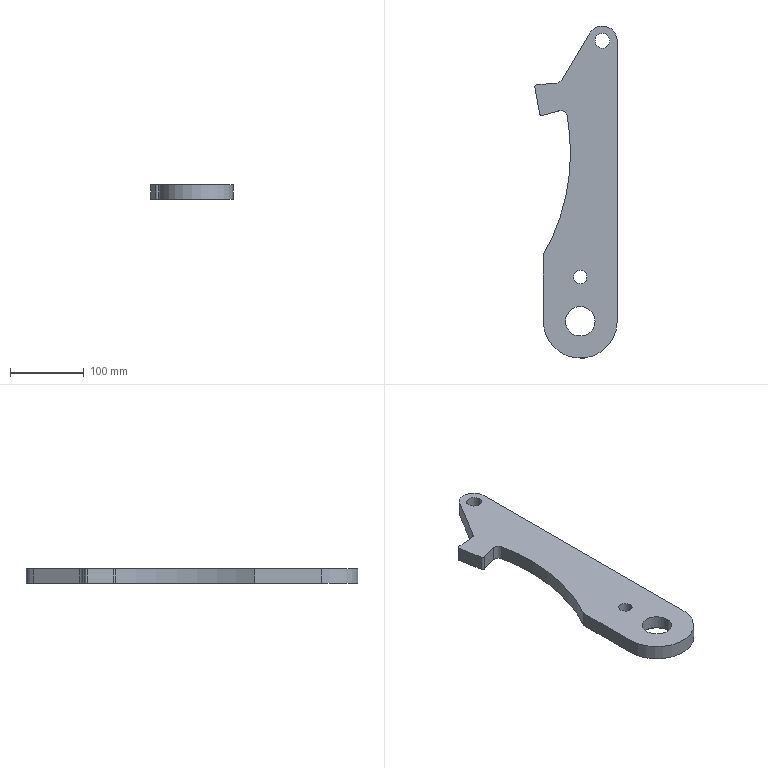Part | SolidWorks | features Fillet 2, Chamfer 1, Extrusion 1 | 1 solid | 24 faces | box 111.471 x 450 x 20 mm | volume 668870 mm3 | cylinder 14 | plane 8 | cone 2 | commonest cylinder face diameters 6 x3 20 x3 40 x3 18 x2 16 x1 100 x1
STEP:
#1=CARTESIAN_POINT('',(20.,0.,2.5));
#2=VERTEX_POINT('',#1);
#3=CARTESIAN_POINT('',(-20.,0.,2.5));
#4=VERTEX_POINT('',#3);
#5=CARTESIAN_POINT('',(0.,0.,2.5));
#6=DIRECTION('',(0.,0.,-1.));
#7=DIRECTION('',(1.,0.,0.));
#8=AXIS2_PLACEMENT_3D('',#5,#6,#7);
#9=CIRCLE('',#8,20.);
#10=EDGE_CURVE('',#2,#4,#9,.T.);
#11=ORIENTED_EDGE('',*,*,#10,.F.);
#12=CARTESIAN_POINT('',(22.5,0.,0.));
#13=VERTEX_POINT('',#12);
#14=CARTESIAN_POINT('',(22.5,0.,0.));
#15=DIRECTION('',(0.7071,0.,-0.7071));
#16=VECTOR('',#15,1000.);
#17=LINE('',#14,#16);
#18=EDGE_CURVE('',#2,#13,#17,.T.);
#19=ORIENTED_EDGE('',*,*,#18,.T.);
#20=CARTESIAN_POINT('',(-22.5,0.,0.));
#21=VERTEX_POINT('',#20);
#22=CARTESIAN_POINT('',(0.,0.,0.));
#23=DIRECTION('',(0.,0.,1.));
#24=DIRECTION('',(1.,0.,0.));
#25=AXIS2_PLACEMENT_3D('',#22,#23,#24);
#26=CIRCLE('',#25,22.5);
#27=EDGE_CURVE('',#21,#13,#26,.T.);
#28=ORIENTED_EDGE('',*,*,#27,.F.);
#29=CARTESIAN_POINT('',(-22.5,0.,0.));
#30=DIRECTION('',(-0.7071,0.,-0.7071));
#31=VECTOR('',#30,1000.);
#32=LINE('',#29,#31);
#33=EDGE_CURVE('',#4,#21,#32,.T.);
#34=ORIENTED_EDGE('',*,*,#33,.F.);
#35=EDGE_LOOP('',(#11,#19,#28,#34));
#36=FACE_OUTER_BOUND('',#35,.T.);
#37=CARTESIAN_POINT('',(0.,0.,0.));
#38=DIRECTION('',(0.,0.,-1.));
#39=DIRECTION('',(-1.,0.,0.));
#40=AXIS2_PLACEMENT_3D('',#37,#38,#39);
#41=CONICAL_SURFACE('',#40,22.5,0.7854);
#42=ADVANCED_FACE('',(#36),#41,.F.);
#43=CARTESIAN_POINT('',(-61.471,317.304,20.));
#44=VERTEX_POINT('',#43);
#45=CARTESIAN_POINT('',(-61.424,316.777,20.));
#46=VERTEX_POINT('',#45);
#47=CARTESIAN_POINT('',(-58.471,317.304,20.));
#48=DIRECTION('',(0.,0.,1.));
#49=DIRECTION('',(1.,0.,0.));
#50=AXIS2_PLACEMENT_3D('',#47,#48,#49);
#51=CIRCLE('',#50,3.);
#52=EDGE_CURVE('',#44,#46,#51,.T.);
#53=ORIENTED_EDGE('',*,*,#52,.F.);
#54=CARTESIAN_POINT('',(-61.471,317.304,0.));
#55=VERTEX_POINT('',#54);
#56=CARTESIAN_POINT('',(-61.471,317.304,20.));
#57=DIRECTION('',(0.,0.,-1.));
#58=VECTOR('',#57,1000.);
#59=LINE('',#56,#58);
#60=EDGE_CURVE('',#44,#55,#59,.T.);
#61=ORIENTED_EDGE('',*,*,#60,.T.);
#62=CARTESIAN_POINT('',(-61.424,316.777,0.));
#63=VERTEX_POINT('',#62);
#64=CARTESIAN_POINT('',(-58.471,317.304,0.));
#65=DIRECTION('',(0.,0.,-1.));
#66=DIRECTION('',(1.,0.,0.));
#67=AXIS2_PLACEMENT_3D('',#64,#65,#66);
#68=CIRCLE('',#67,3.);
#69=EDGE_CURVE('',#63,#55,#68,.T.);
#70=ORIENTED_EDGE('',*,*,#69,.F.);
#71=CARTESIAN_POINT('',(-61.424,316.777,20.));
#72=DIRECTION('',(0.,0.,-1.));
#73=VECTOR('',#72,1000.);
#74=LINE('',#71,#73);
#75=EDGE_CURVE('',#46,#63,#74,.T.);
#76=ORIENTED_EDGE('',*,*,#75,.F.);
#77=EDGE_LOOP('',(#53,#61,#70,#76));
#78=FACE_OUTER_BOUND('',#77,.T.);
#79=CARTESIAN_POINT('',(-58.471,317.304,20.));
#80=DIRECTION('',(0.,0.,-1.));
#81=DIRECTION('',(-1.,0.,0.));
#82=AXIS2_PLACEMENT_3D('',#79,#80,#81);
#83=CYLINDRICAL_SURFACE('',#82,3.);
#84=ADVANCED_FACE('',(#78),#83,.T.);
#85=CARTESIAN_POINT('',(-20.,0.,20.));
#86=VERTEX_POINT('',#85);
#87=CARTESIAN_POINT('',(20.,0.,20.));
#88=VERTEX_POINT('',#87);
#89=CARTESIAN_POINT('',(0.,0.,20.));
#90=DIRECTION('',(0.,0.,1.));
#91=DIRECTION('',(1.,0.,0.));
#92=AXIS2_PLACEMENT_3D('',#89,#90,#91);
#93=CIRCLE('',#92,20.);
#94=EDGE_CURVE('',#86,#88,#93,.T.);
#95=ORIENTED_EDGE('',*,*,#94,.T.);
#96=CARTESIAN_POINT('',(20.,0.,20.));
#97=DIRECTION('',(0.,0.,-1.));
#98=VECTOR('',#97,1000.);
#99=LINE('',#96,#98);
#100=EDGE_CURVE('',#88,#2,#99,.T.);
#101=ORIENTED_EDGE('',*,*,#100,.T.);
#102=ORIENTED_EDGE('',*,*,#10,.T.);
#103=CARTESIAN_POINT('',(-20.,0.,20.));
#104=DIRECTION('',(0.,0.,-1.));
#105=VECTOR('',#104,1000.);
#106=LINE('',#103,#105);
#107=EDGE_CURVE('',#86,#4,#106,.T.);
#108=ORIENTED_EDGE('',*,*,#107,.F.);
#109=EDGE_LOOP('',(#95,#101,#102,#108));
#110=FACE_OUTER_BOUND('',#109,.T.);
#111=CARTESIAN_POINT('',(0.,0.,20.));
#112=DIRECTION('',(0.,0.,-1.));
#113=DIRECTION('',(-1.,0.,0.));
#114=AXIS2_PLACEMENT_3D('',#111,#112,#113);
#115=CYLINDRICAL_SURFACE('',#114,20.);
#116=ADVANCED_FACE('',(#110),#115,.F.);
#117=CARTESIAN_POINT('',(-9.,60.,20.));
#118=VERTEX_POINT('',#117);
#119=CARTESIAN_POINT('',(9.,60.,20.));
#120=VERTEX_POINT('',#119);
#121=CARTESIAN_POINT('',(0.,60.,20.));
#122=DIRECTION('',(0.,0.,1.));
#123=DIRECTION('',(1.,0.,0.));
#124=AXIS2_PLACEMENT_3D('',#121,#122,#123);
#125=CIRCLE('',#124,9.);
#126=EDGE_CURVE('',#118,#120,#125,.T.);
#127=ORIENTED_EDGE('',*,*,#126,.T.);
#128=CARTESIAN_POINT('',(9.,60.,0.));
#129=VERTEX_POINT('',#128);
#130=CARTESIAN_POINT('',(9.,60.,20.));
#131=DIRECTION('',(0.,0.,-1.));
#132=VECTOR('',#131,1000.);
#133=LINE('',#130,#132);
#134=EDGE_CURVE('',#120,#129,#133,.T.);
#135=ORIENTED_EDGE('',*,*,#134,.T.);
#136=CARTESIAN_POINT('',(-9.,60.,0.));
#137=VERTEX_POINT('',#136);
#138=CARTESIAN_POINT('',(0.,60.,0.));
#139=DIRECTION('',(0.,0.,1.));
#140=DIRECTION('',(1.,0.,0.));
#141=AXIS2_PLACEMENT_3D('',#138,#139,#140);
#142=CIRCLE('',#141,9.);
#143=EDGE_CURVE('',#137,#129,#142,.T.);
#144=ORIENTED_EDGE('',*,*,#143,.F.);
#145=CARTESIAN_POINT('',(-9.,60.,20.));
#146=DIRECTION('',(0.,0.,-1.));
#147=VECTOR('',#146,1000.);
#148=LINE('',#145,#147);
#149=EDGE_CURVE('',#118,#137,#148,.T.);
#150=ORIENTED_EDGE('',*,*,#149,.F.);
#151=EDGE_LOOP('',(#127,#135,#144,#150));
#152=FACE_OUTER_BOUND('',#151,.T.);
#153=CARTESIAN_POINT('',(0.,60.,20.));
#154=DIRECTION('',(0.,0.,-1.));
#155=DIRECTION('',(-1.,0.,0.));
#156=AXIS2_PLACEMENT_3D('',#153,#154,#155);
#157=CYLINDRICAL_SURFACE('',#156,9.);
#158=ADVANCED_FACE('',(#152),#157,.F.);
#159=CARTESIAN_POINT('',(20.,380.,20.));
#160=VERTEX_POINT('',#159);
#161=CARTESIAN_POINT('',(40.,380.,20.));
#162=VERTEX_POINT('',#161);
#163=CARTESIAN_POINT('',(30.,380.,20.));
#164=DIRECTION('',(0.,0.,1.));
#165=DIRECTION('',(1.,0.,0.));
#166=AXIS2_PLACEMENT_3D('',#163,#164,#165);
#167=CIRCLE('',#166,10.);
#168=EDGE_CURVE('',#160,#162,#167,.T.);
#169=ORIENTED_EDGE('',*,*,#168,.T.);
#170=CARTESIAN_POINT('',(40.,380.,0.));
#171=VERTEX_POINT('',#170);
#172=CARTESIAN_POINT('',(40.,380.,20.));
#173=DIRECTION('',(0.,0.,-1.));
#174=VECTOR('',#173,1000.);
#175=LINE('',#172,#174);
#176=EDGE_CURVE('',#162,#171,#175,.T.);
#177=ORIENTED_EDGE('',*,*,#176,.T.);
#178=CARTESIAN_POINT('',(20.,380.,0.));
#179=VERTEX_POINT('',#178);
#180=CARTESIAN_POINT('',(30.,380.,0.));
#181=DIRECTION('',(0.,0.,1.));
#182=DIRECTION('',(1.,0.,0.));
#183=AXIS2_PLACEMENT_3D('',#180,#181,#182);
#184=CIRCLE('',#183,10.);
#185=EDGE_CURVE('',#179,#171,#184,.T.);
#186=ORIENTED_EDGE('',*,*,#185,.F.);
#187=CARTESIAN_POINT('',(20.,380.,20.));
#188=DIRECTION('',(0.,0.,-1.));
#189=VECTOR('',#188,1000.);
#190=LINE('',#187,#189);
#191=EDGE_CURVE('',#160,#179,#190,.T.);
#192=ORIENTED_EDGE('',*,*,#191,.F.);
#193=EDGE_LOOP('',(#169,#177,#186,#192));
#194=FACE_OUTER_BOUND('',#193,.T.);
#195=CARTESIAN_POINT('',(30.,380.,20.));
#196=DIRECTION('',(0.,0.,-1.));
#197=DIRECTION('',(-1.,0.,0.));
#198=AXIS2_PLACEMENT_3D('',#195,#196,#197);
#199=CYLINDRICAL_SURFACE('',#198,10.);
#200=ADVANCED_FACE('',(#194),#199,.F.);
#201=ORIENTED_EDGE('',*,*,#126,.F.);
#202=CARTESIAN_POINT('',(0.,60.,20.));
#203=DIRECTION('',(0.,0.,1.));
#204=DIRECTION('',(1.,0.,0.));
#205=AXIS2_PLACEMENT_3D('',#202,#203,#204);
#206=CIRCLE('',#205,9.);
#207=EDGE_CURVE('',#120,#118,#206,.T.);
#208=ORIENTED_EDGE('',*,*,#207,.F.);
#209=EDGE_LOOP('',(#201,#208));
#210=FACE_BOUND('',#209,.T.);
#211=CARTESIAN_POINT('',(12.815,390.232,20.));
#212=VERTEX_POINT('',#211);
#213=CARTESIAN_POINT('',(-24.527,327.514,20.));
#214=VERTEX_POINT('',#213);
#215=CARTESIAN_POINT('',(-27.14,323.126,20.));
#216=DIRECTION('',(-0.5116,-0.8592,0.));
#217=VECTOR('',#216,1000.);
#218=LINE('',#215,#217);
#219=EDGE_CURVE('',#212,#214,#218,.T.);
#220=ORIENTED_EDGE('',*,*,#219,.T.);
#221=CARTESIAN_POINT('',(-32.226,322.67,20.));
#222=VERTEX_POINT('',#221);
#223=CARTESIAN_POINT('',(-33.12,332.63,20.));
#224=DIRECTION('',(0.,0.,-1.));
#225=DIRECTION('',(1.,0.,0.));
#226=AXIS2_PLACEMENT_3D('',#223,#224,#225);
#227=CIRCLE('',#226,10.);
#228=EDGE_CURVE('',#214,#222,#227,.T.);
#229=ORIENTED_EDGE('',*,*,#228,.T.);
#230=CARTESIAN_POINT('',(-58.739,320.292,20.));
#231=VERTEX_POINT('',#230);
#232=CARTESIAN_POINT('',(-62.,320.,20.));
#233=DIRECTION('',(-0.996,-0.08932,0.));
#234=VECTOR('',#233,1000.);
#235=LINE('',#232,#234);
#236=EDGE_CURVE('',#222,#231,#235,.T.);
#237=ORIENTED_EDGE('',*,*,#236,.T.);
#238=CARTESIAN_POINT('',(-58.471,317.304,20.));
#239=DIRECTION('',(0.,0.,1.));
#240=DIRECTION('',(1.,0.,0.));
#241=AXIS2_PLACEMENT_3D('',#238,#239,#240);
#242=CIRCLE('',#241,3.);
#243=EDGE_CURVE('',#231,#44,#242,.T.);
#244=ORIENTED_EDGE('',*,*,#243,.T.);
#245=ORIENTED_EDGE('',*,*,#52,.T.);
#246=CARTESIAN_POINT('',(-55.076,281.223,20.));
#247=VERTEX_POINT('',#246);
#248=CARTESIAN_POINT('',(-54.5,278.,20.));
#249=DIRECTION('',(0.1758,-0.9844,0.));
#250=VECTOR('',#249,1000.);
#251=LINE('',#248,#250);
#252=EDGE_CURVE('',#46,#247,#251,.T.);
#253=ORIENTED_EDGE('',*,*,#252,.T.);
#254=CARTESIAN_POINT('',(-51.339,278.854,20.));
#255=VERTEX_POINT('',#254);
#256=CARTESIAN_POINT('',(-52.122,281.75,20.));
#257=DIRECTION('',(0.,0.,1.));
#258=DIRECTION('',(1.,0.,0.));
#259=AXIS2_PLACEMENT_3D('',#256,#257,#258);
#260=CIRCLE('',#259,3.);
#261=EDGE_CURVE('',#247,#255,#260,.T.);
#262=ORIENTED_EDGE('',*,*,#261,.T.);
#263=CARTESIAN_POINT('',(-27.765,285.226,20.));
#264=VERTEX_POINT('',#263);
#265=CARTESIAN_POINT('',(-54.5,278.,20.));
#266=DIRECTION('',(0.9654,0.2609,0.));
#267=VECTOR('',#266,1000.);
#268=LINE('',#265,#267);
#269=EDGE_CURVE('',#255,#264,#268,.T.);
#270=ORIENTED_EDGE('',*,*,#269,.T.);
#271=CARTESIAN_POINT('',(-17.808,278.94,20.));
#272=VERTEX_POINT('',#271);
#273=CARTESIAN_POINT('',(-25.678,277.503,20.));
#274=DIRECTION('',(0.,0.,-1.));
#275=DIRECTION('',(1.,0.,0.));
#276=AXIS2_PLACEMENT_3D('',#273,#274,#275);
#277=CIRCLE('',#276,8.);
#278=EDGE_CURVE('',#264,#272,#277,.T.);
#279=ORIENTED_EDGE('',*,*,#278,.T.);
#280=CARTESIAN_POINT('',(-50.,90.,20.));
#281=VERTEX_POINT('',#280);
#282=CARTESIAN_POINT('',(-293.256,228.659,20.));
#283=DIRECTION('',(0.,0.,-1.));
#284=DIRECTION('',(1.,0.,0.));
#285=AXIS2_PLACEMENT_3D('',#282,#283,#284);
#286=CIRCLE('',#285,280.);
#287=EDGE_CURVE('',#272,#281,#286,.T.);
#288=ORIENTED_EDGE('',*,*,#287,.T.);
#289=CARTESIAN_POINT('',(-50.,0.,20.));
#290=VERTEX_POINT('',#289);
#291=CARTESIAN_POINT('',(-50.,0.,20.));
#292=DIRECTION('',(0.,-1.,0.));
#293=VECTOR('',#292,1000.);
#294=LINE('',#291,#293);
#295=EDGE_CURVE('',#281,#290,#294,.T.);
#296=ORIENTED_EDGE('',*,*,#295,.T.);
#297=CARTESIAN_POINT('',(50.,0.,20.));
#298=VERTEX_POINT('',#297);
#299=CARTESIAN_POINT('',(0.,0.,20.));
#300=DIRECTION('',(0.,0.,1.));
#301=DIRECTION('',(1.,0.,0.));
#302=AXIS2_PLACEMENT_3D('',#299,#300,#301);
#303=CIRCLE('',#302,50.);
#304=EDGE_CURVE('',#290,#298,#303,.T.);
#305=ORIENTED_EDGE('',*,*,#304,.T.);
#306=CARTESIAN_POINT('',(50.,380.,20.));
#307=VERTEX_POINT('',#306);
#308=CARTESIAN_POINT('',(50.,0.,20.));
#309=DIRECTION('',(0.,1.,0.));
#310=VECTOR('',#309,1000.);
#311=LINE('',#308,#310);
#312=EDGE_CURVE('',#298,#307,#311,.T.);
#313=ORIENTED_EDGE('',*,*,#312,.T.);
#314=CARTESIAN_POINT('',(30.,380.,20.));
#315=DIRECTION('',(0.,0.,1.));
#316=DIRECTION('',(1.,0.,0.));
#317=AXIS2_PLACEMENT_3D('',#314,#315,#316);
#318=CIRCLE('',#317,20.);
#319=EDGE_CURVE('',#307,#212,#318,.T.);
#320=ORIENTED_EDGE('',*,*,#319,.T.);
#321=EDGE_LOOP('',(#220,#229,#237,#244,#245,#253,#262,#270,#279,#288,#296,#305,#313,#320));
#322=FACE_OUTER_BOUND('',#321,.T.);
#323=ORIENTED_EDGE('',*,*,#168,.F.);
#324=CARTESIAN_POINT('',(30.,380.,20.));
#325=DIRECTION('',(0.,0.,1.));
#326=DIRECTION('',(1.,0.,0.));
#327=AXIS2_PLACEMENT_3D('',#324,#325,#326);
#328=CIRCLE('',#327,10.);
#329=EDGE_CURVE('',#162,#160,#328,.T.);
#330=ORIENTED_EDGE('',*,*,#329,.F.);
#331=EDGE_LOOP('',(#323,#330));
#332=FACE_BOUND('',#331,.T.);
#333=ORIENTED_EDGE('',*,*,#94,.F.);
#334=CARTESIAN_POINT('',(0.,0.,20.));
#335=DIRECTION('',(0.,0.,1.));
#336=DIRECTION('',(1.,0.,0.));
#337=AXIS2_PLACEMENT_3D('',#334,#335,#336);
#338=CIRCLE('',#337,20.);
#339=EDGE_CURVE('',#88,#86,#338,.T.);
#340=ORIENTED_EDGE('',*,*,#339,.F.);
#341=EDGE_LOOP('',(#333,#340));
#342=FACE_BOUND('',#341,.T.);
#343=CARTESIAN_POINT('',(0.,0.,20.));
#344=DIRECTION('',(0.,0.,1.));
#345=DIRECTION('',(1.,0.,0.));
#346=AXIS2_PLACEMENT_3D('',#343,#344,#345);
#347=PLANE('',#346);
#348=ADVANCED_FACE('',(#210,#322,#332,#342),#347,.T.);
#349=ORIENTED_EDGE('',*,*,#27,.T.);
#350=CARTESIAN_POINT('',(0.,0.,0.));
#351=DIRECTION('',(0.,0.,1.));
#352=DIRECTION('',(1.,0.,0.));
#353=AXIS2_PLACEMENT_3D('',#350,#351,#352);
#354=CIRCLE('',#353,22.5);
#355=EDGE_CURVE('',#13,#21,#354,.T.);
#356=ORIENTED_EDGE('',*,*,#355,.T.);
#357=EDGE_LOOP('',(#349,#356));
#358=FACE_BOUND('',#357,.T.);
#359=ORIENTED_EDGE('',*,*,#143,.T.);
#360=CARTESIAN_POINT('',(0.,60.,0.));
#361=DIRECTION('',(0.,0.,1.));
#362=DIRECTION('',(1.,0.,0.));
#363=AXIS2_PLACEMENT_3D('',#360,#361,#362);
#364=CIRCLE('',#363,9.);
#365=EDGE_CURVE('',#129,#137,#364,.T.);
#366=ORIENTED_EDGE('',*,*,#365,.T.);
#367=EDGE_LOOP('',(#359,#366));
#368=FACE_BOUND('',#367,.T.);
#369=CARTESIAN_POINT('',(-55.076,281.223,0.));
#370=VERTEX_POINT('',#369);
#371=CARTESIAN_POINT('',(-54.5,278.,0.));
#372=DIRECTION('',(0.1758,-0.9844,0.));
#373=VECTOR('',#372,1000.);
#374=LINE('',#371,#373);
#375=EDGE_CURVE('',#63,#370,#374,.T.);
#376=ORIENTED_EDGE('',*,*,#375,.F.);
#377=ORIENTED_EDGE('',*,*,#69,.T.);
#378=CARTESIAN_POINT('',(-58.739,320.292,0.));
#379=VERTEX_POINT('',#378);
#380=CARTESIAN_POINT('',(-58.471,317.304,0.));
#381=DIRECTION('',(0.,0.,-1.));
#382=DIRECTION('',(1.,0.,0.));
#383=AXIS2_PLACEMENT_3D('',#380,#381,#382);
#384=CIRCLE('',#383,3.);
#385=EDGE_CURVE('',#55,#379,#384,.T.);
#386=ORIENTED_EDGE('',*,*,#385,.T.);
#387=CARTESIAN_POINT('',(-32.226,322.67,0.));
#388=VERTEX_POINT('',#387);
#389=CARTESIAN_POINT('',(-62.,320.,0.));
#390=DIRECTION('',(-0.996,-0.08932,0.));
#391=VECTOR('',#390,1000.);
#392=LINE('',#389,#391);
#393=EDGE_CURVE('',#388,#379,#392,.T.);
#394=ORIENTED_EDGE('',*,*,#393,.F.);
#395=CARTESIAN_POINT('',(-24.527,327.514,0.));
#396=VERTEX_POINT('',#395);
#397=CARTESIAN_POINT('',(-33.12,332.63,0.));
#398=DIRECTION('',(0.,0.,1.));
#399=DIRECTION('',(1.,0.,0.));
#400=AXIS2_PLACEMENT_3D('',#397,#398,#399);
#401=CIRCLE('',#400,10.);
#402=EDGE_CURVE('',#388,#396,#401,.T.);
#403=ORIENTED_EDGE('',*,*,#402,.T.);
#404=CARTESIAN_POINT('',(12.815,390.232,0.));
#405=VERTEX_POINT('',#404);
#406=CARTESIAN_POINT('',(-27.14,323.126,0.));
#407=DIRECTION('',(-0.5116,-0.8592,0.));
#408=VECTOR('',#407,1000.);
#409=LINE('',#406,#408);
#410=EDGE_CURVE('',#405,#396,#409,.T.);
#411=ORIENTED_EDGE('',*,*,#410,.F.);
#412=CARTESIAN_POINT('',(50.,380.,0.));
#413=VERTEX_POINT('',#412);
#414=CARTESIAN_POINT('',(30.,380.,0.));
#415=DIRECTION('',(0.,0.,1.));
#416=DIRECTION('',(1.,0.,0.));
#417=AXIS2_PLACEMENT_3D('',#414,#415,#416);
#418=CIRCLE('',#417,20.);
#419=EDGE_CURVE('',#413,#405,#418,.T.);
#420=ORIENTED_EDGE('',*,*,#419,.F.);
#421=CARTESIAN_POINT('',(50.,0.,0.));
#422=VERTEX_POINT('',#421);
#423=CARTESIAN_POINT('',(50.,0.,0.));
#424=DIRECTION('',(0.,1.,0.));
#425=VECTOR('',#424,1000.);
#426=LINE('',#423,#425);
#427=EDGE_CURVE('',#422,#413,#426,.T.);
#428=ORIENTED_EDGE('',*,*,#427,.F.);
#429=CARTESIAN_POINT('',(-50.,0.,0.));
#430=VERTEX_POINT('',#429);
#431=CARTESIAN_POINT('',(0.,0.,0.));
#432=DIRECTION('',(0.,0.,1.));
#433=DIRECTION('',(1.,0.,0.));
#434=AXIS2_PLACEMENT_3D('',#431,#432,#433);
#435=CIRCLE('',#434,50.);
#436=EDGE_CURVE('',#430,#422,#435,.T.);
#437=ORIENTED_EDGE('',*,*,#436,.F.);
#438=CARTESIAN_POINT('',(-50.,90.,0.));
#439=VERTEX_POINT('',#438);
#440=CARTESIAN_POINT('',(-50.,0.,0.));
#441=DIRECTION('',(0.,-1.,0.));
#442=VECTOR('',#441,1000.);
#443=LINE('',#440,#442);
#444=EDGE_CURVE('',#439,#430,#443,.T.);
#445=ORIENTED_EDGE('',*,*,#444,.F.);
#446=CARTESIAN_POINT('',(-17.808,278.94,0.));
#447=VERTEX_POINT('',#446);
#448=CARTESIAN_POINT('',(-293.256,228.659,0.));
#449=DIRECTION('',(0.,0.,-1.));
#450=DIRECTION('',(1.,0.,0.));
#451=AXIS2_PLACEMENT_3D('',#448,#449,#450);
#452=CIRCLE('',#451,280.);
#453=EDGE_CURVE('',#447,#439,#452,.T.);
#454=ORIENTED_EDGE('',*,*,#453,.F.);
#455=CARTESIAN_POINT('',(-27.765,285.226,0.));
#456=VERTEX_POINT('',#455);
#457=CARTESIAN_POINT('',(-25.678,277.503,0.));
#458=DIRECTION('',(0.,0.,-1.));
#459=DIRECTION('',(1.,0.,0.));
#460=AXIS2_PLACEMENT_3D('',#457,#458,#459);
#461=CIRCLE('',#460,8.);
#462=EDGE_CURVE('',#456,#447,#461,.T.);
#463=ORIENTED_EDGE('',*,*,#462,.F.);
#464=CARTESIAN_POINT('',(-51.339,278.854,0.));
#465=VERTEX_POINT('',#464);
#466=CARTESIAN_POINT('',(-54.5,278.,0.));
#467=DIRECTION('',(0.9654,0.2609,0.));
#468=VECTOR('',#467,1000.);
#469=LINE('',#466,#468);
#470=EDGE_CURVE('',#465,#456,#469,.T.);
#471=ORIENTED_EDGE('',*,*,#470,.F.);
#472=CARTESIAN_POINT('',(-52.122,281.75,0.));
#473=DIRECTION('',(0.,0.,-1.));
#474=DIRECTION('',(1.,0.,0.));
#475=AXIS2_PLACEMENT_3D('',#472,#473,#474);
#476=CIRCLE('',#475,3.);
#477=EDGE_CURVE('',#465,#370,#476,.T.);
#478=ORIENTED_EDGE('',*,*,#477,.T.);
#479=EDGE_LOOP('',(#376,#377,#386,#394,#403,#411,#420,#428,#437,#445,#454,#463,#471,#478));
#480=FACE_OUTER_BOUND('',#479,.T.);
#481=ORIENTED_EDGE('',*,*,#185,.T.);
#482=CARTESIAN_POINT('',(30.,380.,0.));
#483=DIRECTION('',(0.,0.,1.));
#484=DIRECTION('',(1.,0.,0.));
#485=AXIS2_PLACEMENT_3D('',#482,#483,#484);
#486=CIRCLE('',#485,10.);
#487=EDGE_CURVE('',#171,#179,#486,.T.);
#488=ORIENTED_EDGE('',*,*,#487,.T.);
#489=EDGE_LOOP('',(#481,#488));
#490=FACE_BOUND('',#489,.T.);
#491=CARTESIAN_POINT('',(0.,0.,0.));
#492=DIRECTION('',(0.,0.,1.));
#493=DIRECTION('',(1.,0.,0.));
#494=AXIS2_PLACEMENT_3D('',#491,#492,#493);
#495=PLANE('',#494);
#496=ADVANCED_FACE('',(#358,#368,#480,#490),#495,.F.);
#497=ORIENTED_EDGE('',*,*,#436,.T.);
#498=CARTESIAN_POINT('',(50.,0.,20.));
#499=DIRECTION('',(0.,0.,-1.));
#500=VECTOR('',#499,1000.);
#501=LINE('',#498,#500);
#502=EDGE_CURVE('',#298,#422,#501,.T.);
#503=ORIENTED_EDGE('',*,*,#502,.F.);
#504=ORIENTED_EDGE('',*,*,#304,.F.);
#505=CARTESIAN_POINT('',(-50.,0.,20.));
#506=DIRECTION('',(0.,0.,-1.));
#507=VECTOR('',#506,1000.);
#508=LINE('',#505,#507);
#509=EDGE_CURVE('',#290,#430,#508,.T.);
#510=ORIENTED_EDGE('',*,*,#509,.T.);
#511=EDGE_LOOP('',(#497,#503,#504,#510));
#512=FACE_OUTER_BOUND('',#511,.T.);
#513=CARTESIAN_POINT('',(0.,0.,20.));
#514=DIRECTION('',(0.,0.,-1.));
#515=DIRECTION('',(-1.,0.,0.));
#516=AXIS2_PLACEMENT_3D('',#513,#514,#515);
#517=CYLINDRICAL_SURFACE('',#516,50.);
#518=ADVANCED_FACE('',(#512),#517,.T.);
#519=ORIENTED_EDGE('',*,*,#427,.T.);
#520=CARTESIAN_POINT('',(50.,380.,20.));
#521=DIRECTION('',(0.,0.,-1.));
#522=VECTOR('',#521,1000.);
#523=LINE('',#520,#522);
#524=EDGE_CURVE('',#307,#413,#523,.T.);
#525=ORIENTED_EDGE('',*,*,#524,.F.);
#526=ORIENTED_EDGE('',*,*,#312,.F.);
#527=ORIENTED_EDGE('',*,*,#502,.T.);
#528=EDGE_LOOP('',(#519,#525,#526,#527));
#529=FACE_OUTER_BOUND('',#528,.T.);
#530=CARTESIAN_POINT('',(50.,0.,20.));
#531=DIRECTION('',(-1.,0.,0.));
#532=DIRECTION('',(0.,0.,1.));
#533=AXIS2_PLACEMENT_3D('',#530,#531,#532);
#534=PLANE('',#533);
#535=ADVANCED_FACE('',(#529),#534,.F.);
#536=ORIENTED_EDGE('',*,*,#419,.T.);
#537=CARTESIAN_POINT('',(12.815,390.232,20.));
#538=DIRECTION('',(0.,0.,-1.));
#539=VECTOR('',#538,1000.);
#540=LINE('',#537,#539);
#541=EDGE_CURVE('',#212,#405,#540,.T.);
#542=ORIENTED_EDGE('',*,*,#541,.F.);
#543=ORIENTED_EDGE('',*,*,#319,.F.);
#544=ORIENTED_EDGE('',*,*,#524,.T.);
#545=EDGE_LOOP('',(#536,#542,#543,#544));
#546=FACE_OUTER_BOUND('',#545,.T.);
#547=CARTESIAN_POINT('',(30.,380.,20.));
#548=DIRECTION('',(0.,0.,-1.));
#549=DIRECTION('',(-1.,0.,0.));
#550=AXIS2_PLACEMENT_3D('',#547,#548,#549);
#551=CYLINDRICAL_SURFACE('',#550,20.);
#552=ADVANCED_FACE('',(#546),#551,.T.);
#553=ORIENTED_EDGE('',*,*,#410,.T.);
#554=CARTESIAN_POINT('',(-24.527,327.514,20.));
#555=DIRECTION('',(0.,0.,1.));
#556=VECTOR('',#555,1000.);
#557=LINE('',#554,#556);
#558=EDGE_CURVE('',#396,#214,#557,.T.);
#559=ORIENTED_EDGE('',*,*,#558,.T.);
#560=ORIENTED_EDGE('',*,*,#219,.F.);
#561=ORIENTED_EDGE('',*,*,#541,.T.);
#562=EDGE_LOOP('',(#553,#559,#560,#561));
#563=FACE_OUTER_BOUND('',#562,.T.);
#564=CARTESIAN_POINT('',(-27.14,323.126,20.));
#565=DIRECTION('',(0.8592,-0.5116,0.));
#566=DIRECTION('',(0.5116,0.8592,0.));
#567=AXIS2_PLACEMENT_3D('',#564,#565,#566);
#568=PLANE('',#567);
#569=ADVANCED_FACE('',(#563),#568,.F.);
#570=ORIENTED_EDGE('',*,*,#236,.F.);
#571=CARTESIAN_POINT('',(-32.226,322.67,0.));
#572=DIRECTION('',(0.,0.,-1.));
#573=VECTOR('',#572,1000.);
#574=LINE('',#571,#573);
#575=EDGE_CURVE('',#222,#388,#574,.T.);
#576=ORIENTED_EDGE('',*,*,#575,.T.);
#577=ORIENTED_EDGE('',*,*,#393,.T.);
#578=CARTESIAN_POINT('',(-58.739,320.292,20.));
#579=DIRECTION('',(0.,0.,1.));
#580=VECTOR('',#579,1000.);
#581=LINE('',#578,#580);
#582=EDGE_CURVE('',#379,#231,#581,.T.);
#583=ORIENTED_EDGE('',*,*,#582,.T.);
#584=EDGE_LOOP('',(#570,#576,#577,#583));
#585=FACE_OUTER_BOUND('',#584,.T.);
#586=CARTESIAN_POINT('',(-62.,320.,20.));
#587=DIRECTION('',(0.08932,-0.996,0.));
#588=DIRECTION('',(0.996,0.08932,0.));
#589=AXIS2_PLACEMENT_3D('',#586,#587,#588);
#590=PLANE('',#589);
#591=ADVANCED_FACE('',(#585),#590,.F.);
#592=ORIENTED_EDGE('',*,*,#252,.F.);
#593=ORIENTED_EDGE('',*,*,#75,.T.);
#594=ORIENTED_EDGE('',*,*,#375,.T.);
#595=CARTESIAN_POINT('',(-55.076,281.223,20.));
#596=DIRECTION('',(0.,0.,1.));
#597=VECTOR('',#596,1000.);
#598=LINE('',#595,#597);
#599=EDGE_CURVE('',#370,#247,#598,.T.);
#600=ORIENTED_EDGE('',*,*,#599,.T.);
#601=EDGE_LOOP('',(#592,#593,#594,#600));
#602=FACE_OUTER_BOUND('',#601,.T.);
#603=CARTESIAN_POINT('',(-54.5,278.,20.));
#604=DIRECTION('',(0.9844,0.1758,0.));
#605=DIRECTION('',(-0.1758,0.9844,0.));
#606=AXIS2_PLACEMENT_3D('',#603,#604,#605);
#607=PLANE('',#606);
#608=ADVANCED_FACE('',(#602),#607,.F.);
#609=ORIENTED_EDGE('',*,*,#269,.F.);
#610=CARTESIAN_POINT('',(-51.339,278.854,20.));
#611=DIRECTION('',(0.,0.,-1.));
#612=VECTOR('',#611,1000.);
#613=LINE('',#610,#612);
#614=EDGE_CURVE('',#255,#465,#613,.T.);
#615=ORIENTED_EDGE('',*,*,#614,.T.);
#616=ORIENTED_EDGE('',*,*,#470,.T.);
#617=CARTESIAN_POINT('',(-27.765,285.226,20.));
#618=DIRECTION('',(0.,0.,-1.));
#619=VECTOR('',#618,1000.);
#620=LINE('',#617,#619);
#621=EDGE_CURVE('',#264,#456,#620,.T.);
#622=ORIENTED_EDGE('',*,*,#621,.F.);
#623=EDGE_LOOP('',(#609,#615,#616,#622));
#624=FACE_OUTER_BOUND('',#623,.T.);
#625=CARTESIAN_POINT('',(-54.5,278.,20.));
#626=DIRECTION('',(-0.2609,0.9654,0.));
#627=DIRECTION('',(-0.9654,-0.2609,0.));
#628=AXIS2_PLACEMENT_3D('',#625,#626,#627);
#629=PLANE('',#628);
#630=ADVANCED_FACE('',(#624),#629,.F.);
#631=ORIENTED_EDGE('',*,*,#462,.T.);
#632=CARTESIAN_POINT('',(-17.808,278.94,20.));
#633=DIRECTION('',(0.,0.,-1.));
#634=VECTOR('',#633,1000.);
#635=LINE('',#632,#634);
#636=EDGE_CURVE('',#272,#447,#635,.T.);
#637=ORIENTED_EDGE('',*,*,#636,.F.);
#638=ORIENTED_EDGE('',*,*,#278,.F.);
#639=ORIENTED_EDGE('',*,*,#621,.T.);
#640=EDGE_LOOP('',(#631,#637,#638,#639));
#641=FACE_OUTER_BOUND('',#640,.T.);
#642=CARTESIAN_POINT('',(-25.678,277.503,20.));
#643=DIRECTION('',(0.,0.,-1.));
#644=DIRECTION('',(-1.,0.,0.));
#645=AXIS2_PLACEMENT_3D('',#642,#643,#644);
#646=CYLINDRICAL_SURFACE('',#645,8.);
#647=ADVANCED_FACE('',(#641),#646,.F.);
#648=ORIENTED_EDGE('',*,*,#453,.T.);
#649=CARTESIAN_POINT('',(-50.,90.,20.));
#650=DIRECTION('',(0.,0.,-1.));
#651=VECTOR('',#650,1000.);
#652=LINE('',#649,#651);
#653=EDGE_CURVE('',#281,#439,#652,.T.);
#654=ORIENTED_EDGE('',*,*,#653,.F.);
#655=ORIENTED_EDGE('',*,*,#287,.F.);
#656=ORIENTED_EDGE('',*,*,#636,.T.);
#657=EDGE_LOOP('',(#648,#654,#655,#656));
#658=FACE_OUTER_BOUND('',#657,.T.);
#659=CARTESIAN_POINT('',(-293.256,228.659,20.));
#660=DIRECTION('',(0.,0.,-1.));
#661=DIRECTION('',(-1.,0.,0.));
#662=AXIS2_PLACEMENT_3D('',#659,#660,#661);
#663=CYLINDRICAL_SURFACE('',#662,280.);
#664=ADVANCED_FACE('',(#658),#663,.F.);
#665=ORIENTED_EDGE('',*,*,#444,.T.);
#666=ORIENTED_EDGE('',*,*,#509,.F.);
#667=ORIENTED_EDGE('',*,*,#295,.F.);
#668=ORIENTED_EDGE('',*,*,#653,.T.);
#669=EDGE_LOOP('',(#665,#666,#667,#668));
#670=FACE_OUTER_BOUND('',#669,.T.);
#671=CARTESIAN_POINT('',(-50.,0.,20.));
#672=DIRECTION('',(1.,0.,0.));
#673=DIRECTION('',(0.,0.,-1.));
#674=AXIS2_PLACEMENT_3D('',#671,#672,#673);
#675=PLANE('',#674);
#676=ADVANCED_FACE('',(#670),#675,.F.);
#677=ORIENTED_EDGE('',*,*,#176,.F.);
#678=ORIENTED_EDGE('',*,*,#329,.T.);
#679=ORIENTED_EDGE('',*,*,#191,.T.);
#680=ORIENTED_EDGE('',*,*,#487,.F.);
#681=EDGE_LOOP('',(#677,#678,#679,#680));
#682=FACE_OUTER_BOUND('',#681,.T.);
#683=CARTESIAN_POINT('',(30.,380.,20.));
#684=DIRECTION('',(0.,0.,-1.));
#685=DIRECTION('',(-1.,0.,0.));
#686=AXIS2_PLACEMENT_3D('',#683,#684,#685);
#687=CYLINDRICAL_SURFACE('',#686,10.);
#688=ADVANCED_FACE('',(#682),#687,.F.);
#689=ORIENTED_EDGE('',*,*,#134,.F.);
#690=ORIENTED_EDGE('',*,*,#207,.T.);
#691=ORIENTED_EDGE('',*,*,#149,.T.);
#692=ORIENTED_EDGE('',*,*,#365,.F.);
#693=EDGE_LOOP('',(#689,#690,#691,#692));
#694=FACE_OUTER_BOUND('',#693,.T.);
#695=CARTESIAN_POINT('',(0.,60.,20.));
#696=DIRECTION('',(0.,0.,-1.));
#697=DIRECTION('',(-1.,0.,0.));
#698=AXIS2_PLACEMENT_3D('',#695,#696,#697);
#699=CYLINDRICAL_SURFACE('',#698,9.);
#700=ADVANCED_FACE('',(#694),#699,.F.);
#701=ORIENTED_EDGE('',*,*,#100,.F.);
#702=ORIENTED_EDGE('',*,*,#339,.T.);
#703=ORIENTED_EDGE('',*,*,#107,.T.);
#704=CARTESIAN_POINT('',(0.,0.,2.5));
#705=DIRECTION('',(0.,0.,-1.));
#706=DIRECTION('',(1.,0.,0.));
#707=AXIS2_PLACEMENT_3D('',#704,#705,#706);
#708=CIRCLE('',#707,20.);
#709=EDGE_CURVE('',#4,#2,#708,.T.);
#710=ORIENTED_EDGE('',*,*,#709,.T.);
#711=EDGE_LOOP('',(#701,#702,#703,#710));
#712=FACE_OUTER_BOUND('',#711,.T.);
#713=CARTESIAN_POINT('',(0.,0.,20.));
#714=DIRECTION('',(0.,0.,-1.));
#715=DIRECTION('',(-1.,0.,0.));
#716=AXIS2_PLACEMENT_3D('',#713,#714,#715);
#717=CYLINDRICAL_SURFACE('',#716,20.);
#718=ADVANCED_FACE('',(#712),#717,.F.);
#719=ORIENTED_EDGE('',*,*,#60,.F.);
#720=ORIENTED_EDGE('',*,*,#243,.F.);
#721=ORIENTED_EDGE('',*,*,#582,.F.);
#722=ORIENTED_EDGE('',*,*,#385,.F.);
#723=EDGE_LOOP('',(#719,#720,#721,#722));
#724=FACE_OUTER_BOUND('',#723,.T.);
#725=CARTESIAN_POINT('',(-58.471,317.304,20.));
#726=DIRECTION('',(0.,0.,-1.));
#727=DIRECTION('',(-1.,0.,0.));
#728=AXIS2_PLACEMENT_3D('',#725,#726,#727);
#729=CYLINDRICAL_SURFACE('',#728,3.);
#730=ADVANCED_FACE('',(#724),#729,.T.);
#731=ORIENTED_EDGE('',*,*,#261,.F.);
#732=ORIENTED_EDGE('',*,*,#599,.F.);
#733=ORIENTED_EDGE('',*,*,#477,.F.);
#734=ORIENTED_EDGE('',*,*,#614,.F.);
#735=EDGE_LOOP('',(#731,#732,#733,#734));
#736=FACE_OUTER_BOUND('',#735,.T.);
#737=CARTESIAN_POINT('',(-52.122,281.75,20.));
#738=DIRECTION('',(0.,0.,-1.));
#739=DIRECTION('',(-1.,0.,0.));
#740=AXIS2_PLACEMENT_3D('',#737,#738,#739);
#741=CYLINDRICAL_SURFACE('',#740,3.);
#742=ADVANCED_FACE('',(#736),#741,.T.);
#743=ORIENTED_EDGE('',*,*,#228,.F.);
#744=ORIENTED_EDGE('',*,*,#558,.F.);
#745=ORIENTED_EDGE('',*,*,#402,.F.);
#746=ORIENTED_EDGE('',*,*,#575,.F.);
#747=EDGE_LOOP('',(#743,#744,#745,#746));
#748=FACE_OUTER_BOUND('',#747,.T.);
#749=CARTESIAN_POINT('',(-33.12,332.63,20.));
#750=DIRECTION('',(0.,0.,1.));
#751=DIRECTION('',(1.,0.,0.));
#752=AXIS2_PLACEMENT_3D('',#749,#750,#751);
#753=CYLINDRICAL_SURFACE('',#752,10.);
#754=ADVANCED_FACE('',(#748),#753,.F.);
#755=ORIENTED_EDGE('',*,*,#18,.F.);
#756=ORIENTED_EDGE('',*,*,#709,.F.);
#757=ORIENTED_EDGE('',*,*,#33,.T.);
#758=ORIENTED_EDGE('',*,*,#355,.F.);
#759=EDGE_LOOP('',(#755,#756,#757,#758));
#760=FACE_OUTER_BOUND('',#759,.T.);
#761=CARTESIAN_POINT('',(0.,0.,0.));
#762=DIRECTION('',(0.,0.,-1.));
#763=DIRECTION('',(-1.,0.,0.));
#764=AXIS2_PLACEMENT_3D('',#761,#762,#763);
#765=CONICAL_SURFACE('',#764,22.5,0.7854);
#766=ADVANCED_FACE('',(#760),#765,.F.);
#767=CLOSED_SHELL('',(#42,#84,#116,#158,#200,#348,#496,#518,#535,#552,#569,#591,#608,#630,#647,#664,#676,#688,#700,#718,#730,#742,#754,#766));
#768=MANIFOLD_SOLID_BREP('',#767);
#769=CARTESIAN_POINT('',(0.,0.,0.));
#770=DIRECTION('',(0.,0.,1.));
#771=DIRECTION('',(1.,0.,0.));
#772=AXIS2_PLACEMENT_3D('',#769,#770,#771);
#773=(LENGTH_UNIT()NAMED_UNIT(*)SI_UNIT(.MILLI.,.METRE.));
#774=UNCERTAINTY_MEASURE_WITH_UNIT(LENGTH_MEASURE(0.00001),#773,'','');
#775=(NAMED_UNIT(*)PLANE_ANGLE_UNIT()SI_UNIT($,.RADIAN.));
#776=(NAMED_UNIT(*)SI_UNIT($,.STERADIAN.)SOLID_ANGLE_UNIT());
#777=(GEOMETRIC_REPRESENTATION_CONTEXT(3)GLOBAL_UNCERTAINTY_ASSIGNED_CONTEXT((#774))GLOBAL_UNIT_ASSIGNED_CONTEXT((#773,#775,#776))REPRESENTATION_CONTEXT('',''));
#778=ADVANCED_BREP_SHAPE_REPRESENTATION('',(#768,#772),#777);